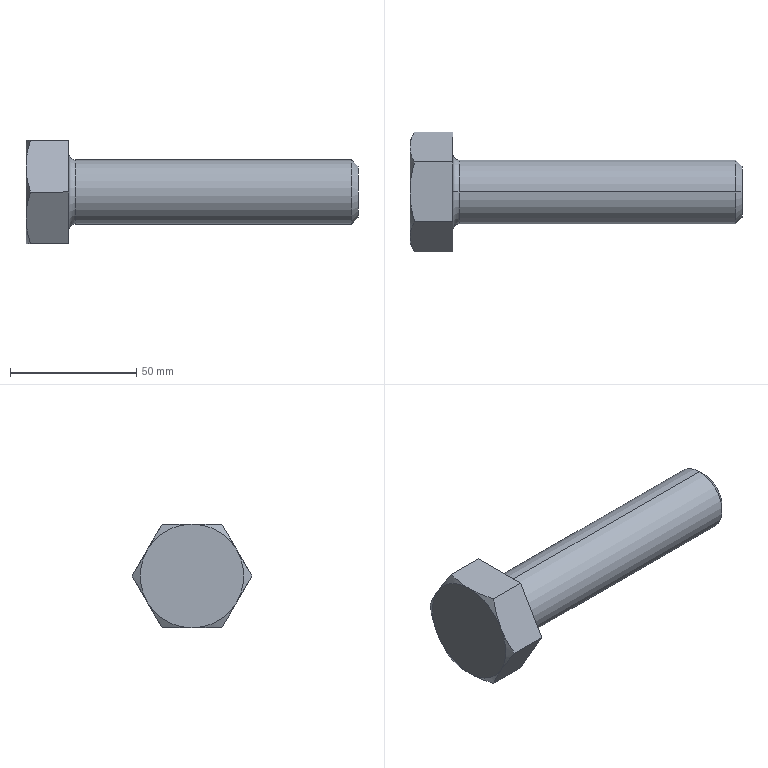Part | SolidWorks | features RevCut 4, Chamfer 1, Extrusion 1, Fillet 1, LPattern 1, Revolution 1 | 1 solid | 21 faces | box 131.3 x 47.343 x 41 mm | volume 82460 mm3 | plane 9 | cone 8 | torus 2 | cylinder 2 | commonest cylinder face diameters 25.4 x2
STEP:
#1=CARTESIAN_POINT('',(19.4,0.,12.7));
#2=VERTEX_POINT('',#1);
#3=CARTESIAN_POINT('',(19.4,0.,-12.7));
#4=VERTEX_POINT('',#3);
#5=CARTESIAN_POINT('',(19.4,0.,0.));
#6=DIRECTION('',(1.,0.,0.));
#7=DIRECTION('',(0.,0.,-1.));
#8=AXIS2_PLACEMENT_3D('',#5,#6,#7);
#9=CIRCLE('',#8,12.7);
#10=EDGE_CURVE('',#2,#4,#9,.T.);
#11=ORIENTED_EDGE('',*,*,#10,.F.);
#12=CARTESIAN_POINT('',(17.,0.,15.1));
#13=VERTEX_POINT('',#12);
#14=CARTESIAN_POINT('',(19.4,0.,15.1));
#15=DIRECTION('',(0.,1.,0.));
#16=DIRECTION('',(0.,0.,1.));
#17=AXIS2_PLACEMENT_3D('',#14,#15,#16);
#18=CIRCLE('',#17,2.4);
#19=EDGE_CURVE('',#2,#13,#18,.T.);
#20=ORIENTED_EDGE('',*,*,#19,.T.);
#21=CARTESIAN_POINT('',(17.,0.,-15.1));
#22=VERTEX_POINT('',#21);
#23=CARTESIAN_POINT('',(17.,0.,0.));
#24=DIRECTION('',(-1.,0.,0.));
#25=DIRECTION('',(0.,0.,-1.));
#26=AXIS2_PLACEMENT_3D('',#23,#24,#25);
#27=CIRCLE('',#26,15.1);
#28=EDGE_CURVE('',#22,#13,#27,.T.);
#29=ORIENTED_EDGE('',*,*,#28,.F.);
#30=CARTESIAN_POINT('',(19.4,0.,-15.1));
#31=DIRECTION('',(0.,-1.,0.));
#32=DIRECTION('',(1.,0.,0.));
#33=AXIS2_PLACEMENT_3D('',#30,#31,#32);
#34=CIRCLE('',#33,2.4);
#35=EDGE_CURVE('',#4,#22,#34,.T.);
#36=ORIENTED_EDGE('',*,*,#35,.F.);
#37=EDGE_LOOP('',(#11,#20,#29,#36));
#38=FACE_OUTER_BOUND('',#37,.T.);
#39=CARTESIAN_POINT('',(19.4,0.,0.));
#40=DIRECTION('',(1.,0.,0.));
#41=DIRECTION('',(0.,0.,-1.));
#42=AXIS2_PLACEMENT_3D('',#39,#40,#41);
#43=TOROIDAL_SURFACE('',#42,15.1,2.4);
#44=ADVANCED_FACE('',(#38),#43,.F.);
#45=CARTESIAN_POINT('',(131.3,0.,-10.2));
#46=VERTEX_POINT('',#45);
#47=CARTESIAN_POINT('',(131.3,0.,10.2));
#48=VERTEX_POINT('',#47);
#49=CARTESIAN_POINT('',(131.3,0.,0.));
#50=DIRECTION('',(1.,0.,0.));
#51=DIRECTION('',(0.,0.,1.));
#52=AXIS2_PLACEMENT_3D('',#49,#50,#51);
#53=CIRCLE('',#52,10.2);
#54=EDGE_CURVE('',#46,#48,#53,.T.);
#55=ORIENTED_EDGE('',*,*,#54,.F.);
#56=CARTESIAN_POINT('',(128.8,0.,-12.7));
#57=VERTEX_POINT('',#56);
#58=CARTESIAN_POINT('',(128.8,0.,-12.7));
#59=DIRECTION('',(-0.7071,0.,-0.7071));
#60=VECTOR('',#59,1000.);
#61=LINE('',#58,#60);
#62=EDGE_CURVE('',#46,#57,#61,.T.);
#63=ORIENTED_EDGE('',*,*,#62,.T.);
#64=CARTESIAN_POINT('',(128.8,0.,12.7));
#65=VERTEX_POINT('',#64);
#66=CARTESIAN_POINT('',(128.8,0.,0.));
#67=DIRECTION('',(-1.,0.,0.));
#68=DIRECTION('',(0.,0.,1.));
#69=AXIS2_PLACEMENT_3D('',#66,#67,#68);
#70=CIRCLE('',#69,12.7);
#71=EDGE_CURVE('',#65,#57,#70,.T.);
#72=ORIENTED_EDGE('',*,*,#71,.F.);
#73=CARTESIAN_POINT('',(128.8,0.,12.7));
#74=DIRECTION('',(-0.7071,0.,0.7071));
#75=VECTOR('',#74,1000.);
#76=LINE('',#73,#75);
#77=EDGE_CURVE('',#48,#65,#76,.T.);
#78=ORIENTED_EDGE('',*,*,#77,.F.);
#79=EDGE_LOOP('',(#55,#63,#72,#78));
#80=FACE_OUTER_BOUND('',#79,.T.);
#81=CARTESIAN_POINT('',(128.8,0.,0.));
#82=DIRECTION('',(-1.,0.,0.));
#83=DIRECTION('',(0.,0.,1.));
#84=AXIS2_PLACEMENT_3D('',#81,#82,#83);
#85=CONICAL_SURFACE('',#84,12.7,0.7854);
#86=ADVANCED_FACE('',(#80),#85,.T.);
#87=ORIENTED_EDGE('',*,*,#71,.T.);
#88=CARTESIAN_POINT('',(0.,0.,-12.7));
#89=DIRECTION('',(-1.,0.,0.));
#90=VECTOR('',#89,1000.);
#91=LINE('',#88,#90);
#92=EDGE_CURVE('',#57,#4,#91,.T.);
#93=ORIENTED_EDGE('',*,*,#92,.T.);
#94=CARTESIAN_POINT('',(19.4,0.,0.));
#95=DIRECTION('',(1.,0.,0.));
#96=DIRECTION('',(0.,0.,-1.));
#97=AXIS2_PLACEMENT_3D('',#94,#95,#96);
#98=CIRCLE('',#97,12.7);
#99=EDGE_CURVE('',#4,#2,#98,.T.);
#100=ORIENTED_EDGE('',*,*,#99,.T.);
#101=CARTESIAN_POINT('',(0.,0.,12.7));
#102=DIRECTION('',(-1.,0.,0.));
#103=VECTOR('',#102,1000.);
#104=LINE('',#101,#103);
#105=EDGE_CURVE('',#65,#2,#104,.T.);
#106=ORIENTED_EDGE('',*,*,#105,.F.);
#107=EDGE_LOOP('',(#87,#93,#100,#106));
#108=FACE_OUTER_BOUND('',#107,.T.);
#109=CARTESIAN_POINT('',(0.,0.,0.));
#110=DIRECTION('',(-1.,0.,0.));
#111=DIRECTION('',(0.,0.,1.));
#112=AXIS2_PLACEMENT_3D('',#109,#110,#111);
#113=CYLINDRICAL_SURFACE('',#112,12.7);
#114=ADVANCED_FACE('',(#108),#113,.T.);
#115=CARTESIAN_POINT('',(1.831,23.671,0.));
#116=VERTEX_POINT('',#115);
#117=CARTESIAN_POINT('',(0.,17.754,-10.25));
#118=VERTEX_POINT('',#117);
#119=CARTESIAN_POINT('',(1.831,23.671,0.));
#120=CARTESIAN_POINT('',(1.272,22.703,-1.677));
#121=CARTESIAN_POINT('',(0.8116,21.728,-3.366));
#122=CARTESIAN_POINT('',(0.1745,19.757,-6.779));
#123=CARTESIAN_POINT('',(0.,18.762,-8.504));
#124=CARTESIAN_POINT('',(0.,17.754,-10.25));
#125=B_SPLINE_CURVE_WITH_KNOTS('',3,(#119,#120,#121,#122,#123,#124),.UNSPECIFIED.,.F.,.F.,(4,2,4),(0.000000238,0.005988,0.01198),.UNSPECIFIED.);
#126=EDGE_CURVE('',#116,#118,#125,.T.);
#127=ORIENTED_EDGE('',*,*,#126,.F.);
#128=CARTESIAN_POINT('',(17.,23.671,0.));
#129=VERTEX_POINT('',#128);
#130=CARTESIAN_POINT('',(17.,23.671,0.));
#131=DIRECTION('',(-1.,0.,0.));
#132=VECTOR('',#131,1000.);
#133=LINE('',#130,#132);
#134=EDGE_CURVE('',#129,#116,#133,.T.);
#135=ORIENTED_EDGE('',*,*,#134,.F.);
#136=CARTESIAN_POINT('',(17.,11.836,-20.5));
#137=VERTEX_POINT('',#136);
#138=CARTESIAN_POINT('',(17.,11.836,-20.5));
#139=DIRECTION('',(0.,0.5,0.866));
#140=VECTOR('',#139,1000.);
#141=LINE('',#138,#140);
#142=EDGE_CURVE('',#137,#129,#141,.T.);
#143=ORIENTED_EDGE('',*,*,#142,.F.);
#144=CARTESIAN_POINT('',(1.831,11.836,-20.5));
#145=VERTEX_POINT('',#144);
#146=CARTESIAN_POINT('',(17.,11.836,-20.5));
#147=DIRECTION('',(-1.,0.,0.));
#148=VECTOR('',#147,1000.);
#149=LINE('',#146,#148);
#150=EDGE_CURVE('',#137,#145,#149,.T.);
#151=ORIENTED_EDGE('',*,*,#150,.T.);
#152=CARTESIAN_POINT('',(0.,17.754,-10.25));
#153=CARTESIAN_POINT('',(0.,17.502,-10.685));
#154=CARTESIAN_POINT('',(0.01074,17.25,-11.122));
#155=CARTESIAN_POINT('',(0.05334,16.748,-11.992));
#156=CARTESIAN_POINT('',(0.08515,16.497,-12.426));
#157=CARTESIAN_POINT('',(0.2108,15.749,-13.722));
#158=CARTESIAN_POINT('',(0.3348,15.253,-14.581));
#159=CARTESIAN_POINT('',(0.8132,13.775,-17.141));
#160=CARTESIAN_POINT('',(1.273,12.801,-18.827));
#161=CARTESIAN_POINT('',(1.831,11.836,-20.5));
#162=B_SPLINE_CURVE_WITH_KNOTS('',3,(#152,#153,#154,#155,#156,#157,#158,#159,#160,#161),.UNSPECIFIED.,.F.,.F.,(4,2,2,2,4),(0.01198,0.01347,0.01496,0.01794,0.02391),.UNSPECIFIED.);
#163=EDGE_CURVE('',#118,#145,#162,.T.);
#164=ORIENTED_EDGE('',*,*,#163,.F.);
#165=EDGE_LOOP('',(#127,#135,#143,#151,#164));
#166=FACE_OUTER_BOUND('',#165,.T.);
#167=CARTESIAN_POINT('',(17.,11.836,-20.5));
#168=DIRECTION('',(0.,-0.866,0.5));
#169=DIRECTION('',(0.,-0.5,-0.866));
#170=AXIS2_PLACEMENT_3D('',#167,#168,#169);
#171=PLANE('',#170);
#172=ADVANCED_FACE('',(#166),#171,.F.);
#173=CARTESIAN_POINT('',(1.831,11.836,20.5));
#174=VERTEX_POINT('',#173);
#175=CARTESIAN_POINT('',(0.,17.754,10.25));
#176=VERTEX_POINT('',#175);
#177=CARTESIAN_POINT('',(1.831,11.836,20.5));
#178=CARTESIAN_POINT('',(1.272,12.804,18.823));
#179=CARTESIAN_POINT('',(0.8116,13.779,17.134));
#180=CARTESIAN_POINT('',(0.1745,15.75,13.721));
#181=CARTESIAN_POINT('',(0.,16.745,11.996));
#182=CARTESIAN_POINT('',(0.,17.754,10.25));
#183=B_SPLINE_CURVE_WITH_KNOTS('',3,(#177,#178,#179,#180,#181,#182),.UNSPECIFIED.,.F.,.F.,(4,2,4),(0.000000238,0.005988,0.01198),.UNSPECIFIED.);
#184=EDGE_CURVE('',#174,#176,#183,.T.);
#185=ORIENTED_EDGE('',*,*,#184,.F.);
#186=CARTESIAN_POINT('',(17.,11.836,20.5));
#187=VERTEX_POINT('',#186);
#188=CARTESIAN_POINT('',(17.,11.836,20.5));
#189=DIRECTION('',(-1.,0.,0.));
#190=VECTOR('',#189,1000.);
#191=LINE('',#188,#190);
#192=EDGE_CURVE('',#187,#174,#191,.T.);
#193=ORIENTED_EDGE('',*,*,#192,.F.);
#194=CARTESIAN_POINT('',(17.,23.671,0.));
#195=DIRECTION('',(0.,-0.5,0.866));
#196=VECTOR('',#195,1000.);
#197=LINE('',#194,#196);
#198=EDGE_CURVE('',#129,#187,#197,.T.);
#199=ORIENTED_EDGE('',*,*,#198,.F.);
#200=ORIENTED_EDGE('',*,*,#134,.T.);
#201=CARTESIAN_POINT('',(0.,17.754,10.25));
#202=CARTESIAN_POINT('',(0.,18.005,9.815));
#203=CARTESIAN_POINT('',(0.01074,18.257,9.378));
#204=CARTESIAN_POINT('',(0.05334,18.759,8.508));
#205=CARTESIAN_POINT('',(0.08515,19.01,8.074));
#206=CARTESIAN_POINT('',(0.2108,19.758,6.778));
#207=CARTESIAN_POINT('',(0.3348,20.254,5.919));
#208=CARTESIAN_POINT('',(0.8132,21.732,3.359));
#209=CARTESIAN_POINT('',(1.273,22.706,1.673));
#210=CARTESIAN_POINT('',(1.831,23.671,0.));
#211=B_SPLINE_CURVE_WITH_KNOTS('',3,(#201,#202,#203,#204,#205,#206,#207,#208,#209,#210),.UNSPECIFIED.,.F.,.F.,(4,2,2,2,4),(0.01198,0.01347,0.01496,0.01794,0.02391),.UNSPECIFIED.);
#212=EDGE_CURVE('',#176,#116,#211,.T.);
#213=ORIENTED_EDGE('',*,*,#212,.F.);
#214=EDGE_LOOP('',(#185,#193,#199,#200,#213));
#215=FACE_OUTER_BOUND('',#214,.T.);
#216=CARTESIAN_POINT('',(17.,23.671,0.));
#217=DIRECTION('',(0.,-0.866,-0.5));
#218=DIRECTION('',(0.,0.5,-0.866));
#219=AXIS2_PLACEMENT_3D('',#216,#217,#218);
#220=PLANE('',#219);
#221=ADVANCED_FACE('',(#215),#220,.F.);
#222=CARTESIAN_POINT('',(1.831,-11.836,20.5));
#223=VERTEX_POINT('',#222);
#224=CARTESIAN_POINT('',(0.,0.,20.5));
#225=VERTEX_POINT('',#224);
#226=CARTESIAN_POINT('',(1.831,-11.836,20.5));
#227=CARTESIAN_POINT('',(1.553,-10.873,20.5));
#228=CARTESIAN_POINT('',(1.297,-9.899,20.5));
#229=CARTESIAN_POINT('',(0.8451,-7.935,20.5));
#230=CARTESIAN_POINT('',(0.6498,-6.951,20.5));
#231=CARTESIAN_POINT('',(0.1721,-3.988,20.5));
#232=CARTESIAN_POINT('',(0.,-2.001,20.5));
#233=CARTESIAN_POINT('',(0.,0.,20.5));
#234=B_SPLINE_CURVE_WITH_KNOTS('',3,(#226,#227,#228,#229,#230,#231,#232,#233),.UNSPECIFIED.,.F.,.F.,(4,2,2,4),(0.02156,0.02456,0.02755,0.03354),.UNSPECIFIED.);
#235=EDGE_CURVE('',#223,#225,#234,.T.);
#236=ORIENTED_EDGE('',*,*,#235,.F.);
#237=CARTESIAN_POINT('',(17.,-11.836,20.5));
#238=VERTEX_POINT('',#237);
#239=CARTESIAN_POINT('',(17.,-11.836,20.5));
#240=DIRECTION('',(-1.,0.,0.));
#241=VECTOR('',#240,1000.);
#242=LINE('',#239,#241);
#243=EDGE_CURVE('',#238,#223,#242,.T.);
#244=ORIENTED_EDGE('',*,*,#243,.F.);
#245=CARTESIAN_POINT('',(17.,11.836,20.5));
#246=DIRECTION('',(0.,-1.,0.));
#247=VECTOR('',#246,1000.);
#248=LINE('',#245,#247);
#249=EDGE_CURVE('',#187,#238,#248,.T.);
#250=ORIENTED_EDGE('',*,*,#249,.F.);
#251=ORIENTED_EDGE('',*,*,#192,.T.);
#252=CARTESIAN_POINT('',(0.,0.,20.5));
#253=CARTESIAN_POINT('',(0.,1.001,20.5));
#254=CARTESIAN_POINT('',(0.04262,2.007,20.5));
#255=CARTESIAN_POINT('',(0.2119,4.022,20.5));
#256=CARTESIAN_POINT('',(0.3373,5.02,20.5));
#257=CARTESIAN_POINT('',(0.8185,7.983,20.5));
#258=CARTESIAN_POINT('',(1.278,9.922,20.5));
#259=CARTESIAN_POINT('',(1.831,11.836,20.5));
#260=B_SPLINE_CURVE_WITH_KNOTS('',3,(#252,#253,#254,#255,#256,#257,#258,#259),.UNSPECIFIED.,.F.,.F.,(4,2,2,4),(0.03354,0.03654,0.03953,0.04553),.UNSPECIFIED.);
#261=EDGE_CURVE('',#225,#174,#260,.T.);
#262=ORIENTED_EDGE('',*,*,#261,.F.);
#263=EDGE_LOOP('',(#236,#244,#250,#251,#262));
#264=FACE_OUTER_BOUND('',#263,.T.);
#265=CARTESIAN_POINT('',(17.,11.836,20.5));
#266=DIRECTION('',(0.,0.,-1.));
#267=DIRECTION('',(0.,1.,0.));
#268=AXIS2_PLACEMENT_3D('',#265,#266,#267);
#269=PLANE('',#268);
#270=ADVANCED_FACE('',(#264),#269,.F.);
#271=CARTESIAN_POINT('',(1.831,-23.671,0.));
#272=VERTEX_POINT('',#271);
#273=CARTESIAN_POINT('',(0.,-17.754,10.25));
#274=VERTEX_POINT('',#273);
#275=CARTESIAN_POINT('',(1.831,-23.671,0.));
#276=CARTESIAN_POINT('',(1.272,-22.703,1.677));
#277=CARTESIAN_POINT('',(0.8116,-21.728,3.366));
#278=CARTESIAN_POINT('',(0.1745,-19.757,6.779));
#279=CARTESIAN_POINT('',(0.,-18.762,8.504));
#280=CARTESIAN_POINT('',(0.,-17.754,10.25));
#281=B_SPLINE_CURVE_WITH_KNOTS('',3,(#275,#276,#277,#278,#279,#280),.UNSPECIFIED.,.F.,.F.,(4,2,4),(0.000000238,0.005988,0.01198),.UNSPECIFIED.);
#282=EDGE_CURVE('',#272,#274,#281,.T.);
#283=ORIENTED_EDGE('',*,*,#282,.F.);
#284=CARTESIAN_POINT('',(17.,-23.671,0.));
#285=VERTEX_POINT('',#284);
#286=CARTESIAN_POINT('',(17.,-23.671,0.));
#287=DIRECTION('',(-1.,0.,0.));
#288=VECTOR('',#287,1000.);
#289=LINE('',#286,#288);
#290=EDGE_CURVE('',#285,#272,#289,.T.);
#291=ORIENTED_EDGE('',*,*,#290,.F.);
#292=CARTESIAN_POINT('',(17.,-23.671,0.));
#293=DIRECTION('',(0.,-0.5,-0.866));
#294=VECTOR('',#293,1000.);
#295=LINE('',#292,#294);
#296=EDGE_CURVE('',#238,#285,#295,.T.);
#297=ORIENTED_EDGE('',*,*,#296,.F.);
#298=ORIENTED_EDGE('',*,*,#243,.T.);
#299=CARTESIAN_POINT('',(0.,-17.754,10.25));
#300=CARTESIAN_POINT('',(0.,-17.502,10.685));
#301=CARTESIAN_POINT('',(0.01074,-17.25,11.122));
#302=CARTESIAN_POINT('',(0.05334,-16.748,11.992));
#303=CARTESIAN_POINT('',(0.08515,-16.497,12.426));
#304=CARTESIAN_POINT('',(0.2108,-15.749,13.722));
#305=CARTESIAN_POINT('',(0.3348,-15.253,14.581));
#306=CARTESIAN_POINT('',(0.8132,-13.775,17.141));
#307=CARTESIAN_POINT('',(1.273,-12.801,18.827));
#308=CARTESIAN_POINT('',(1.831,-11.836,20.5));
#309=B_SPLINE_CURVE_WITH_KNOTS('',3,(#299,#300,#301,#302,#303,#304,#305,#306,#307,#308),.UNSPECIFIED.,.F.,.F.,(4,2,2,2,4),(0.01198,0.01347,0.01496,0.01794,0.02391),.UNSPECIFIED.);
#310=EDGE_CURVE('',#274,#223,#309,.T.);
#311=ORIENTED_EDGE('',*,*,#310,.F.);
#312=EDGE_LOOP('',(#283,#291,#297,#298,#311));
#313=FACE_OUTER_BOUND('',#312,.T.);
#314=CARTESIAN_POINT('',(17.,-23.671,0.));
#315=DIRECTION('',(0.,0.866,-0.5));
#316=DIRECTION('',(0.,0.5,0.866));
#317=AXIS2_PLACEMENT_3D('',#314,#315,#316);
#318=PLANE('',#317);
#319=ADVANCED_FACE('',(#313),#318,.F.);
#320=CARTESIAN_POINT('',(1.831,-11.836,-20.5));
#321=VERTEX_POINT('',#320);
#322=CARTESIAN_POINT('',(0.,-17.754,-10.25));
#323=VERTEX_POINT('',#322);
#324=CARTESIAN_POINT('',(1.831,-11.836,-20.5));
#325=CARTESIAN_POINT('',(1.272,-12.804,-18.823));
#326=CARTESIAN_POINT('',(0.8116,-13.779,-17.134));
#327=CARTESIAN_POINT('',(0.1745,-15.75,-13.721));
#328=CARTESIAN_POINT('',(0.,-16.745,-11.996));
#329=CARTESIAN_POINT('',(0.,-17.754,-10.25));
#330=B_SPLINE_CURVE_WITH_KNOTS('',3,(#324,#325,#326,#327,#328,#329),.UNSPECIFIED.,.F.,.F.,(4,2,4),(0.000000238,0.005988,0.01198),.UNSPECIFIED.);
#331=EDGE_CURVE('',#321,#323,#330,.T.);
#332=ORIENTED_EDGE('',*,*,#331,.F.);
#333=CARTESIAN_POINT('',(17.,-11.836,-20.5));
#334=VERTEX_POINT('',#333);
#335=CARTESIAN_POINT('',(17.,-11.836,-20.5));
#336=DIRECTION('',(-1.,0.,0.));
#337=VECTOR('',#336,1000.);
#338=LINE('',#335,#337);
#339=EDGE_CURVE('',#334,#321,#338,.T.);
#340=ORIENTED_EDGE('',*,*,#339,.F.);
#341=CARTESIAN_POINT('',(17.,-11.836,-20.5));
#342=DIRECTION('',(0.,0.5,-0.866));
#343=VECTOR('',#342,1000.);
#344=LINE('',#341,#343);
#345=EDGE_CURVE('',#285,#334,#344,.T.);
#346=ORIENTED_EDGE('',*,*,#345,.F.);
#347=ORIENTED_EDGE('',*,*,#290,.T.);
#348=CARTESIAN_POINT('',(0.,-17.754,-10.25));
#349=CARTESIAN_POINT('',(0.,-18.005,-9.815));
#350=CARTESIAN_POINT('',(0.01074,-18.257,-9.378));
#351=CARTESIAN_POINT('',(0.05334,-18.759,-8.508));
#352=CARTESIAN_POINT('',(0.08515,-19.01,-8.074));
#353=CARTESIAN_POINT('',(0.2108,-19.758,-6.778));
#354=CARTESIAN_POINT('',(0.3348,-20.254,-5.919));
#355=CARTESIAN_POINT('',(0.8132,-21.732,-3.359));
#356=CARTESIAN_POINT('',(1.273,-22.706,-1.673));
#357=CARTESIAN_POINT('',(1.831,-23.671,0.));
#358=B_SPLINE_CURVE_WITH_KNOTS('',3,(#348,#349,#350,#351,#352,#353,#354,#355,#356,#357),.UNSPECIFIED.,.F.,.F.,(4,2,2,2,4),(0.01198,0.01347,0.01496,0.01794,0.02391),.UNSPECIFIED.);
#359=EDGE_CURVE('',#323,#272,#358,.T.);
#360=ORIENTED_EDGE('',*,*,#359,.F.);
#361=EDGE_LOOP('',(#332,#340,#346,#347,#360));
#362=FACE_OUTER_BOUND('',#361,.T.);
#363=CARTESIAN_POINT('',(17.,-11.836,-20.5));
#364=DIRECTION('',(0.,0.866,0.5));
#365=DIRECTION('',(0.,-0.5,0.866));
#366=AXIS2_PLACEMENT_3D('',#363,#364,#365);
#367=PLANE('',#366);
#368=ADVANCED_FACE('',(#362),#367,.F.);
#369=CARTESIAN_POINT('',(0.,0.,-20.5));
#370=VERTEX_POINT('',#369);
#371=CARTESIAN_POINT('',(1.831,11.836,-20.5));
#372=CARTESIAN_POINT('',(1.278,9.922,-20.5));
#373=CARTESIAN_POINT('',(0.8185,7.983,-20.5));
#374=CARTESIAN_POINT('',(0.3373,5.02,-20.5));
#375=CARTESIAN_POINT('',(0.2119,4.022,-20.5));
#376=CARTESIAN_POINT('',(0.04262,2.007,-20.5));
#377=CARTESIAN_POINT('',(0.,1.001,-20.5));
#378=CARTESIAN_POINT('',(0.,0.,-20.5));
#379=B_SPLINE_CURVE_WITH_KNOTS('',3,(#371,#372,#373,#374,#375,#376,#377,#378),.UNSPECIFIED.,.F.,.F.,(4,2,2,4),(0.0533,0.05929,0.06229,0.06529),.UNSPECIFIED.);
#380=EDGE_CURVE('',#145,#370,#379,.T.);
#381=ORIENTED_EDGE('',*,*,#380,.F.);
#382=ORIENTED_EDGE('',*,*,#150,.F.);
#383=CARTESIAN_POINT('',(17.,11.836,-20.5));
#384=DIRECTION('',(0.,1.,0.));
#385=VECTOR('',#384,1000.);
#386=LINE('',#383,#385);
#387=EDGE_CURVE('',#334,#137,#386,.T.);
#388=ORIENTED_EDGE('',*,*,#387,.F.);
#389=ORIENTED_EDGE('',*,*,#339,.T.);
#390=CARTESIAN_POINT('',(0.,0.,-20.5));
#391=CARTESIAN_POINT('',(0.,-2.001,-20.5));
#392=CARTESIAN_POINT('',(0.1721,-3.988,-20.5));
#393=CARTESIAN_POINT('',(0.6498,-6.951,-20.5));
#394=CARTESIAN_POINT('',(0.8451,-7.935,-20.5));
#395=CARTESIAN_POINT('',(1.297,-9.899,-20.5));
#396=CARTESIAN_POINT('',(1.553,-10.873,-20.5));
#397=CARTESIAN_POINT('',(1.831,-11.836,-20.5));
#398=B_SPLINE_CURVE_WITH_KNOTS('',3,(#390,#391,#392,#393,#394,#395,#396,#397),.UNSPECIFIED.,.F.,.F.,(4,2,2,4),(0.06529,0.07128,0.07428,0.07728),.UNSPECIFIED.);
#399=EDGE_CURVE('',#370,#321,#398,.T.);
#400=ORIENTED_EDGE('',*,*,#399,.F.);
#401=EDGE_LOOP('',(#381,#382,#388,#389,#400));
#402=FACE_OUTER_BOUND('',#401,.T.);
#403=CARTESIAN_POINT('',(17.,11.836,-20.5));
#404=DIRECTION('',(0.,0.,1.));
#405=DIRECTION('',(0.,-1.,0.));
#406=AXIS2_PLACEMENT_3D('',#403,#404,#405);
#407=PLANE('',#406);
#408=ADVANCED_FACE('',(#402),#407,.F.);
#409=ORIENTED_EDGE('',*,*,#28,.T.);
#410=CARTESIAN_POINT('',(17.,0.,0.));
#411=DIRECTION('',(-1.,0.,0.));
#412=DIRECTION('',(0.,0.,-1.));
#413=AXIS2_PLACEMENT_3D('',#410,#411,#412);
#414=CIRCLE('',#413,15.1);
#415=EDGE_CURVE('',#13,#22,#414,.T.);
#416=ORIENTED_EDGE('',*,*,#415,.T.);
#417=EDGE_LOOP('',(#409,#416));
#418=FACE_BOUND('',#417,.T.);
#419=ORIENTED_EDGE('',*,*,#142,.T.);
#420=ORIENTED_EDGE('',*,*,#198,.T.);
#421=ORIENTED_EDGE('',*,*,#249,.T.);
#422=ORIENTED_EDGE('',*,*,#296,.T.);
#423=ORIENTED_EDGE('',*,*,#345,.T.);
#424=ORIENTED_EDGE('',*,*,#387,.T.);
#425=EDGE_LOOP('',(#419,#420,#421,#422,#423,#424));
#426=FACE_OUTER_BOUND('',#425,.T.);
#427=CARTESIAN_POINT('',(17.,23.671,0.));
#428=DIRECTION('',(1.,0.,0.));
#429=DIRECTION('',(0.,0.,-1.));
#430=AXIS2_PLACEMENT_3D('',#427,#428,#429);
#431=PLANE('',#430);
#432=ADVANCED_FACE('',(#418,#426),#431,.T.);
#433=ORIENTED_EDGE('',*,*,#92,.F.);
#434=CARTESIAN_POINT('',(128.8,0.,0.));
#435=DIRECTION('',(-1.,0.,0.));
#436=DIRECTION('',(0.,0.,1.));
#437=AXIS2_PLACEMENT_3D('',#434,#435,#436);
#438=CIRCLE('',#437,12.7);
#439=EDGE_CURVE('',#57,#65,#438,.T.);
#440=ORIENTED_EDGE('',*,*,#439,.T.);
#441=ORIENTED_EDGE('',*,*,#105,.T.);
#442=ORIENTED_EDGE('',*,*,#10,.T.);
#443=EDGE_LOOP('',(#433,#440,#441,#442));
#444=FACE_OUTER_BOUND('',#443,.T.);
#445=CARTESIAN_POINT('',(0.,0.,0.));
#446=DIRECTION('',(-1.,0.,0.));
#447=DIRECTION('',(0.,0.,1.));
#448=AXIS2_PLACEMENT_3D('',#445,#446,#447);
#449=CYLINDRICAL_SURFACE('',#448,12.7);
#450=ADVANCED_FACE('',(#444),#449,.T.);
#451=CARTESIAN_POINT('',(131.3,0.,0.));
#452=DIRECTION('',(1.,0.,0.));
#453=DIRECTION('',(0.,0.,1.));
#454=AXIS2_PLACEMENT_3D('',#451,#452,#453);
#455=CIRCLE('',#454,10.2);
#456=EDGE_CURVE('',#48,#46,#455,.T.);
#457=ORIENTED_EDGE('',*,*,#456,.T.);
#458=ORIENTED_EDGE('',*,*,#54,.T.);
#459=EDGE_LOOP('',(#457,#458));
#460=FACE_OUTER_BOUND('',#459,.T.);
#461=CARTESIAN_POINT('',(131.3,0.,0.));
#462=DIRECTION('',(-1.,0.,0.));
#463=DIRECTION('',(0.,0.,1.));
#464=AXIS2_PLACEMENT_3D('',#461,#462,#463);
#465=PLANE('',#464);
#466=ADVANCED_FACE('',(#460),#465,.F.);
#467=ORIENTED_EDGE('',*,*,#331,.T.);
#468=CARTESIAN_POINT('',(0.,0.,0.));
#469=DIRECTION('',(1.,0.,0.));
#470=DIRECTION('',(0.,0.,-1.));
#471=AXIS2_PLACEMENT_3D('',#468,#469,#470);
#472=CIRCLE('',#471,20.5);
#473=EDGE_CURVE('',#323,#370,#472,.T.);
#474=ORIENTED_EDGE('',*,*,#473,.T.);
#475=ORIENTED_EDGE('',*,*,#399,.T.);
#476=EDGE_LOOP('',(#467,#474,#475));
#477=FACE_OUTER_BOUND('',#476,.T.);
#478=CARTESIAN_POINT('',(0.,0.,0.));
#479=DIRECTION('',(1.,0.,0.));
#480=DIRECTION('',(0.,0.,-1.));
#481=AXIS2_PLACEMENT_3D('',#478,#479,#480);
#482=CONICAL_SURFACE('',#481,20.5,1.047);
#483=ADVANCED_FACE('',(#477),#482,.T.);
#484=ORIENTED_EDGE('',*,*,#282,.T.);
#485=CARTESIAN_POINT('',(0.,0.,0.));
#486=DIRECTION('',(1.,0.,0.));
#487=DIRECTION('',(0.,0.,-1.));
#488=AXIS2_PLACEMENT_3D('',#485,#486,#487);
#489=CIRCLE('',#488,20.5);
#490=EDGE_CURVE('',#274,#323,#489,.T.);
#491=ORIENTED_EDGE('',*,*,#490,.T.);
#492=ORIENTED_EDGE('',*,*,#359,.T.);
#493=EDGE_LOOP('',(#484,#491,#492));
#494=FACE_OUTER_BOUND('',#493,.T.);
#495=CARTESIAN_POINT('',(0.,0.,0.));
#496=DIRECTION('',(1.,0.,0.));
#497=DIRECTION('',(0.,0.,-1.));
#498=AXIS2_PLACEMENT_3D('',#495,#496,#497);
#499=CONICAL_SURFACE('',#498,20.5,1.047);
#500=ADVANCED_FACE('',(#494),#499,.T.);
#501=ORIENTED_EDGE('',*,*,#235,.T.);
#502=CARTESIAN_POINT('',(0.,0.,0.));
#503=DIRECTION('',(1.,0.,0.));
#504=DIRECTION('',(0.,0.,-1.));
#505=AXIS2_PLACEMENT_3D('',#502,#503,#504);
#506=CIRCLE('',#505,20.5);
#507=EDGE_CURVE('',#225,#274,#506,.T.);
#508=ORIENTED_EDGE('',*,*,#507,.T.);
#509=ORIENTED_EDGE('',*,*,#310,.T.);
#510=EDGE_LOOP('',(#501,#508,#509));
#511=FACE_OUTER_BOUND('',#510,.T.);
#512=CARTESIAN_POINT('',(0.,0.,0.));
#513=DIRECTION('',(1.,0.,0.));
#514=DIRECTION('',(0.,0.,-1.));
#515=AXIS2_PLACEMENT_3D('',#512,#513,#514);
#516=CONICAL_SURFACE('',#515,20.5,1.047);
#517=ADVANCED_FACE('',(#511),#516,.T.);
#518=ORIENTED_EDGE('',*,*,#261,.T.);
#519=ORIENTED_EDGE('',*,*,#184,.T.);
#520=CARTESIAN_POINT('',(0.,0.,0.));
#521=DIRECTION('',(-1.,0.,0.));
#522=DIRECTION('',(0.,0.,1.));
#523=AXIS2_PLACEMENT_3D('',#520,#521,#522);
#524=CIRCLE('',#523,20.5);
#525=EDGE_CURVE('',#225,#176,#524,.T.);
#526=ORIENTED_EDGE('',*,*,#525,.F.);
#527=EDGE_LOOP('',(#518,#519,#526));
#528=FACE_OUTER_BOUND('',#527,.T.);
#529=CARTESIAN_POINT('',(0.,0.,0.));
#530=DIRECTION('',(1.,0.,0.));
#531=DIRECTION('',(0.,0.,-1.));
#532=AXIS2_PLACEMENT_3D('',#529,#530,#531);
#533=CONICAL_SURFACE('',#532,20.5,1.047);
#534=ADVANCED_FACE('',(#528),#533,.T.);
#535=ORIENTED_EDGE('',*,*,#212,.T.);
#536=ORIENTED_EDGE('',*,*,#126,.T.);
#537=CARTESIAN_POINT('',(0.,0.,0.));
#538=DIRECTION('',(1.,0.,0.));
#539=DIRECTION('',(0.,0.,-1.));
#540=AXIS2_PLACEMENT_3D('',#537,#538,#539);
#541=CIRCLE('',#540,20.5);
#542=EDGE_CURVE('',#118,#176,#541,.T.);
#543=ORIENTED_EDGE('',*,*,#542,.T.);
#544=EDGE_LOOP('',(#535,#536,#543));
#545=FACE_OUTER_BOUND('',#544,.T.);
#546=CARTESIAN_POINT('',(0.,0.,0.));
#547=DIRECTION('',(1.,0.,0.));
#548=DIRECTION('',(0.,0.,-1.));
#549=AXIS2_PLACEMENT_3D('',#546,#547,#548);
#550=CONICAL_SURFACE('',#549,20.5,1.047);
#551=ADVANCED_FACE('',(#545),#550,.T.);
#552=ORIENTED_EDGE('',*,*,#163,.T.);
#553=ORIENTED_EDGE('',*,*,#380,.T.);
#554=CARTESIAN_POINT('',(0.,0.,0.));
#555=DIRECTION('',(1.,0.,0.));
#556=DIRECTION('',(0.,0.,-1.));
#557=AXIS2_PLACEMENT_3D('',#554,#555,#556);
#558=CIRCLE('',#557,20.5);
#559=EDGE_CURVE('',#370,#118,#558,.T.);
#560=ORIENTED_EDGE('',*,*,#559,.T.);
#561=EDGE_LOOP('',(#552,#553,#560));
#562=FACE_OUTER_BOUND('',#561,.T.);
#563=CARTESIAN_POINT('',(0.,0.,0.));
#564=DIRECTION('',(1.,0.,0.));
#565=DIRECTION('',(0.,0.,-1.));
#566=AXIS2_PLACEMENT_3D('',#563,#564,#565);
#567=CONICAL_SURFACE('',#566,20.5,1.047);
#568=ADVANCED_FACE('',(#562),#567,.T.);
#569=ORIENTED_EDGE('',*,*,#559,.F.);
#570=ORIENTED_EDGE('',*,*,#473,.F.);
#571=ORIENTED_EDGE('',*,*,#490,.F.);
#572=ORIENTED_EDGE('',*,*,#507,.F.);
#573=ORIENTED_EDGE('',*,*,#525,.T.);
#574=ORIENTED_EDGE('',*,*,#542,.F.);
#575=EDGE_LOOP('',(#569,#570,#571,#572,#573,#574));
#576=FACE_OUTER_BOUND('',#575,.T.);
#577=CARTESIAN_POINT('',(0.,23.671,0.));
#578=DIRECTION('',(1.,0.,0.));
#579=DIRECTION('',(0.,0.,-1.));
#580=AXIS2_PLACEMENT_3D('',#577,#578,#579);
#581=PLANE('',#580);
#582=ADVANCED_FACE('',(#576),#581,.F.);
#583=ORIENTED_EDGE('',*,*,#62,.F.);
#584=ORIENTED_EDGE('',*,*,#456,.F.);
#585=ORIENTED_EDGE('',*,*,#77,.T.);
#586=ORIENTED_EDGE('',*,*,#439,.F.);
#587=EDGE_LOOP('',(#583,#584,#585,#586));
#588=FACE_OUTER_BOUND('',#587,.T.);
#589=CARTESIAN_POINT('',(128.8,0.,0.));
#590=DIRECTION('',(-1.,0.,0.));
#591=DIRECTION('',(0.,0.,1.));
#592=AXIS2_PLACEMENT_3D('',#589,#590,#591);
#593=CONICAL_SURFACE('',#592,12.7,0.7854);
#594=ADVANCED_FACE('',(#588),#593,.T.);
#595=ORIENTED_EDGE('',*,*,#19,.F.);
#596=ORIENTED_EDGE('',*,*,#99,.F.);
#597=ORIENTED_EDGE('',*,*,#35,.T.);
#598=ORIENTED_EDGE('',*,*,#415,.F.);
#599=EDGE_LOOP('',(#595,#596,#597,#598));
#600=FACE_OUTER_BOUND('',#599,.T.);
#601=CARTESIAN_POINT('',(19.4,0.,0.));
#602=DIRECTION('',(1.,0.,0.));
#603=DIRECTION('',(0.,0.,-1.));
#604=AXIS2_PLACEMENT_3D('',#601,#602,#603);
#605=TOROIDAL_SURFACE('',#604,15.1,2.4);
#606=ADVANCED_FACE('',(#600),#605,.F.);
#607=CLOSED_SHELL('',(#44,#86,#114,#172,#221,#270,#319,#368,#408,#432,#450,#466,#483,#500,#517,#534,#551,#568,#582,#594,#606));
#608=MANIFOLD_SOLID_BREP('',#607);
#609=CARTESIAN_POINT('',(0.,0.,0.));
#610=DIRECTION('',(0.,0.,1.));
#611=DIRECTION('',(1.,0.,0.));
#612=AXIS2_PLACEMENT_3D('',#609,#610,#611);
#613=(LENGTH_UNIT()NAMED_UNIT(*)SI_UNIT(.MILLI.,.METRE.));
#614=UNCERTAINTY_MEASURE_WITH_UNIT(LENGTH_MEASURE(0.00001),#613,'','');
#615=(NAMED_UNIT(*)PLANE_ANGLE_UNIT()SI_UNIT($,.RADIAN.));
#616=(NAMED_UNIT(*)SI_UNIT($,.STERADIAN.)SOLID_ANGLE_UNIT());
#617=(GEOMETRIC_REPRESENTATION_CONTEXT(3)GLOBAL_UNCERTAINTY_ASSIGNED_CONTEXT((#614))GLOBAL_UNIT_ASSIGNED_CONTEXT((#613,#615,#616))REPRESENTATION_CONTEXT('',''));
#618=ADVANCED_BREP_SHAPE_REPRESENTATION('',(#608,#612),#617);